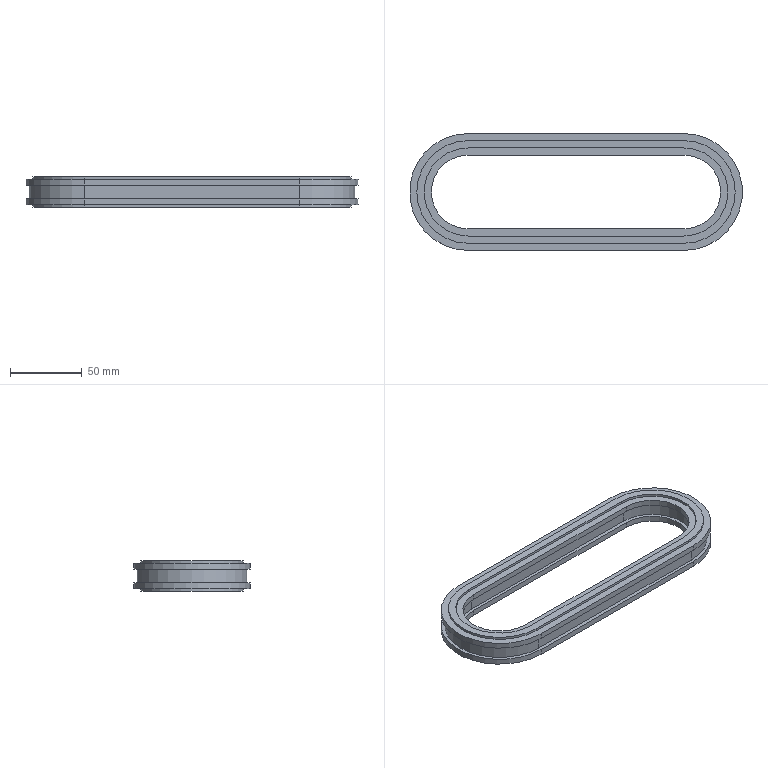Part | STEP file | Roller chain | 1 solid | 50 faces | box 231.346 x 81.346 x 21.082 mm | volume 120087 mm3 | plane 30 | cylinder 20 | commonest cylinder face diameters 51.324 x4 61.255 x4 71.415 x4 81.346 x4 56.175 x2 76.495 x2